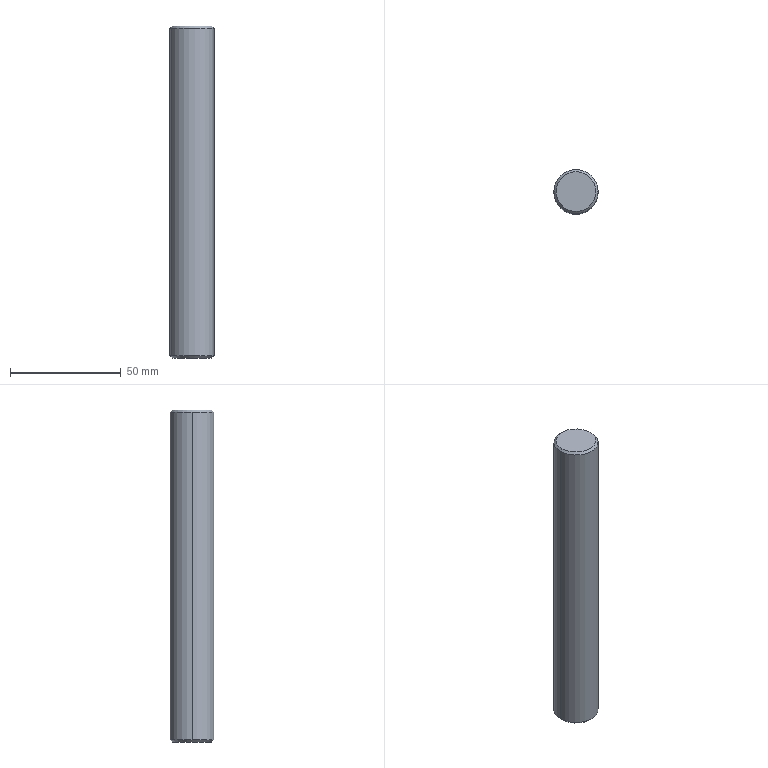Part | SolidWorks | features Chamfer 1, Extrusion 1 | 1 solid | 8 faces | box 20 x 20 x 150 mm | volume 47063 mm3 | cone 4 | cylinder 2 | plane 2 | commonest cylinder face diameters 20 x2
STEP:
#1=CARTESIAN_POINT('',(9.,0.,0.));
#2=VERTEX_POINT('',#1);
#3=CARTESIAN_POINT('',(-9.,0.,0.));
#4=VERTEX_POINT('',#3);
#5=CARTESIAN_POINT('',(0.,0.,0.));
#6=DIRECTION('',(0.,0.,1.));
#7=DIRECTION('',(1.,0.,0.));
#8=AXIS2_PLACEMENT_3D('',#5,#6,#7);
#9=CIRCLE('',#8,9.);
#10=EDGE_CURVE('',#2,#4,#9,.T.);
#11=ORIENTED_EDGE('',*,*,#10,.F.);
#12=CARTESIAN_POINT('',(10.,0.,-1.));
#13=VERTEX_POINT('',#12);
#14=CARTESIAN_POINT('',(9.,0.,0.));
#15=DIRECTION('',(0.7071,0.,-0.7071));
#16=VECTOR('',#15,1000.);
#17=LINE('',#14,#16);
#18=EDGE_CURVE('',#2,#13,#17,.T.);
#19=ORIENTED_EDGE('',*,*,#18,.T.);
#20=CARTESIAN_POINT('',(-10.,0.,-1.));
#21=VERTEX_POINT('',#20);
#22=CARTESIAN_POINT('',(0.,0.,-1.));
#23=DIRECTION('',(0.,0.,-1.));
#24=DIRECTION('',(1.,0.,0.));
#25=AXIS2_PLACEMENT_3D('',#22,#23,#24);
#26=CIRCLE('',#25,10.);
#27=EDGE_CURVE('',#21,#13,#26,.T.);
#28=ORIENTED_EDGE('',*,*,#27,.F.);
#29=CARTESIAN_POINT('',(-9.,0.,0.));
#30=DIRECTION('',(-0.7071,0.,-0.7071));
#31=VECTOR('',#30,1000.);
#32=LINE('',#29,#31);
#33=EDGE_CURVE('',#4,#21,#32,.T.);
#34=ORIENTED_EDGE('',*,*,#33,.F.);
#35=EDGE_LOOP('',(#11,#19,#28,#34));
#36=FACE_OUTER_BOUND('',#35,.T.);
#37=CARTESIAN_POINT('',(0.,0.,0.));
#38=DIRECTION('',(0.,0.,-1.));
#39=DIRECTION('',(-1.,0.,0.));
#40=AXIS2_PLACEMENT_3D('',#37,#38,#39);
#41=CONICAL_SURFACE('',#40,9.,0.7854);
#42=ADVANCED_FACE('',(#36),#41,.T.);
#43=CARTESIAN_POINT('',(-9.,0.,-150.));
#44=VERTEX_POINT('',#43);
#45=CARTESIAN_POINT('',(9.,0.,-150.));
#46=VERTEX_POINT('',#45);
#47=CARTESIAN_POINT('',(0.,0.,-150.));
#48=DIRECTION('',(0.,0.,-1.));
#49=DIRECTION('',(1.,0.,0.));
#50=AXIS2_PLACEMENT_3D('',#47,#48,#49);
#51=CIRCLE('',#50,9.);
#52=EDGE_CURVE('',#44,#46,#51,.T.);
#53=ORIENTED_EDGE('',*,*,#52,.F.);
#54=CARTESIAN_POINT('',(-10.,0.,-149.));
#55=VERTEX_POINT('',#54);
#56=CARTESIAN_POINT('',(-10.,0.,-149.));
#57=DIRECTION('',(-0.7071,0.,0.7071));
#58=VECTOR('',#57,1000.);
#59=LINE('',#56,#58);
#60=EDGE_CURVE('',#44,#55,#59,.T.);
#61=ORIENTED_EDGE('',*,*,#60,.T.);
#62=CARTESIAN_POINT('',(10.,0.,-149.));
#63=VERTEX_POINT('',#62);
#64=CARTESIAN_POINT('',(0.,0.,-149.));
#65=DIRECTION('',(0.,0.,1.));
#66=DIRECTION('',(1.,0.,0.));
#67=AXIS2_PLACEMENT_3D('',#64,#65,#66);
#68=CIRCLE('',#67,10.);
#69=EDGE_CURVE('',#63,#55,#68,.T.);
#70=ORIENTED_EDGE('',*,*,#69,.F.);
#71=CARTESIAN_POINT('',(10.,0.,-149.));
#72=DIRECTION('',(0.7071,0.,0.7071));
#73=VECTOR('',#72,1000.);
#74=LINE('',#71,#73);
#75=EDGE_CURVE('',#46,#63,#74,.T.);
#76=ORIENTED_EDGE('',*,*,#75,.F.);
#77=EDGE_LOOP('',(#53,#61,#70,#76));
#78=FACE_OUTER_BOUND('',#77,.T.);
#79=CARTESIAN_POINT('',(0.,0.,-149.));
#80=DIRECTION('',(0.,0.,1.));
#81=DIRECTION('',(1.,0.,0.));
#82=AXIS2_PLACEMENT_3D('',#79,#80,#81);
#83=CONICAL_SURFACE('',#82,10.,0.7854);
#84=ADVANCED_FACE('',(#78),#83,.T.);
#85=ORIENTED_EDGE('',*,*,#69,.T.);
#86=CARTESIAN_POINT('',(-10.,0.,-150.));
#87=DIRECTION('',(0.,0.,1.));
#88=VECTOR('',#87,1000.);
#89=LINE('',#86,#88);
#90=EDGE_CURVE('',#55,#21,#89,.T.);
#91=ORIENTED_EDGE('',*,*,#90,.T.);
#92=ORIENTED_EDGE('',*,*,#27,.T.);
#93=CARTESIAN_POINT('',(10.,0.,-150.));
#94=DIRECTION('',(0.,0.,1.));
#95=VECTOR('',#94,1000.);
#96=LINE('',#93,#95);
#97=EDGE_CURVE('',#63,#13,#96,.T.);
#98=ORIENTED_EDGE('',*,*,#97,.F.);
#99=EDGE_LOOP('',(#85,#91,#92,#98));
#100=FACE_OUTER_BOUND('',#99,.T.);
#101=CARTESIAN_POINT('',(0.,0.,-150.));
#102=DIRECTION('',(0.,0.,1.));
#103=DIRECTION('',(1.,0.,0.));
#104=AXIS2_PLACEMENT_3D('',#101,#102,#103);
#105=CYLINDRICAL_SURFACE('',#104,10.);
#106=ADVANCED_FACE('',(#100),#105,.T.);
#107=ORIENTED_EDGE('',*,*,#90,.F.);
#108=CARTESIAN_POINT('',(0.,0.,-149.));
#109=DIRECTION('',(0.,0.,1.));
#110=DIRECTION('',(1.,0.,0.));
#111=AXIS2_PLACEMENT_3D('',#108,#109,#110);
#112=CIRCLE('',#111,10.);
#113=EDGE_CURVE('',#55,#63,#112,.T.);
#114=ORIENTED_EDGE('',*,*,#113,.T.);
#115=ORIENTED_EDGE('',*,*,#97,.T.);
#116=CARTESIAN_POINT('',(0.,0.,-1.));
#117=DIRECTION('',(0.,0.,-1.));
#118=DIRECTION('',(1.,0.,0.));
#119=AXIS2_PLACEMENT_3D('',#116,#117,#118);
#120=CIRCLE('',#119,10.);
#121=EDGE_CURVE('',#13,#21,#120,.T.);
#122=ORIENTED_EDGE('',*,*,#121,.T.);
#123=EDGE_LOOP('',(#107,#114,#115,#122));
#124=FACE_OUTER_BOUND('',#123,.T.);
#125=CARTESIAN_POINT('',(0.,0.,-150.));
#126=DIRECTION('',(0.,0.,1.));
#127=DIRECTION('',(1.,0.,0.));
#128=AXIS2_PLACEMENT_3D('',#125,#126,#127);
#129=CYLINDRICAL_SURFACE('',#128,10.);
#130=ADVANCED_FACE('',(#124),#129,.T.);
#131=CARTESIAN_POINT('',(0.,0.,-150.));
#132=DIRECTION('',(0.,0.,-1.));
#133=DIRECTION('',(1.,0.,0.));
#134=AXIS2_PLACEMENT_3D('',#131,#132,#133);
#135=CIRCLE('',#134,9.);
#136=EDGE_CURVE('',#46,#44,#135,.T.);
#137=ORIENTED_EDGE('',*,*,#136,.T.);
#138=ORIENTED_EDGE('',*,*,#52,.T.);
#139=EDGE_LOOP('',(#137,#138));
#140=FACE_OUTER_BOUND('',#139,.T.);
#141=CARTESIAN_POINT('',(0.,0.,-150.));
#142=DIRECTION('',(0.,0.,1.));
#143=DIRECTION('',(1.,0.,0.));
#144=AXIS2_PLACEMENT_3D('',#141,#142,#143);
#145=PLANE('',#144);
#146=ADVANCED_FACE('',(#140),#145,.F.);
#147=CARTESIAN_POINT('',(0.,0.,0.));
#148=DIRECTION('',(0.,0.,1.));
#149=DIRECTION('',(1.,0.,0.));
#150=AXIS2_PLACEMENT_3D('',#147,#148,#149);
#151=CIRCLE('',#150,9.);
#152=EDGE_CURVE('',#4,#2,#151,.T.);
#153=ORIENTED_EDGE('',*,*,#152,.T.);
#154=ORIENTED_EDGE('',*,*,#10,.T.);
#155=EDGE_LOOP('',(#153,#154));
#156=FACE_OUTER_BOUND('',#155,.T.);
#157=CARTESIAN_POINT('',(0.,0.,0.));
#158=DIRECTION('',(0.,0.,1.));
#159=DIRECTION('',(1.,0.,0.));
#160=AXIS2_PLACEMENT_3D('',#157,#158,#159);
#161=PLANE('',#160);
#162=ADVANCED_FACE('',(#156),#161,.T.);
#163=ORIENTED_EDGE('',*,*,#60,.F.);
#164=ORIENTED_EDGE('',*,*,#136,.F.);
#165=ORIENTED_EDGE('',*,*,#75,.T.);
#166=ORIENTED_EDGE('',*,*,#113,.F.);
#167=EDGE_LOOP('',(#163,#164,#165,#166));
#168=FACE_OUTER_BOUND('',#167,.T.);
#169=CARTESIAN_POINT('',(0.,0.,-149.));
#170=DIRECTION('',(0.,0.,1.));
#171=DIRECTION('',(1.,0.,0.));
#172=AXIS2_PLACEMENT_3D('',#169,#170,#171);
#173=CONICAL_SURFACE('',#172,10.,0.7854);
#174=ADVANCED_FACE('',(#168),#173,.T.);
#175=ORIENTED_EDGE('',*,*,#18,.F.);
#176=ORIENTED_EDGE('',*,*,#152,.F.);
#177=ORIENTED_EDGE('',*,*,#33,.T.);
#178=ORIENTED_EDGE('',*,*,#121,.F.);
#179=EDGE_LOOP('',(#175,#176,#177,#178));
#180=FACE_OUTER_BOUND('',#179,.T.);
#181=CARTESIAN_POINT('',(0.,0.,0.));
#182=DIRECTION('',(0.,0.,-1.));
#183=DIRECTION('',(-1.,0.,0.));
#184=AXIS2_PLACEMENT_3D('',#181,#182,#183);
#185=CONICAL_SURFACE('',#184,9.,0.7854);
#186=ADVANCED_FACE('',(#180),#185,.T.);
#187=CLOSED_SHELL('',(#42,#84,#106,#130,#146,#162,#174,#186));
#188=MANIFOLD_SOLID_BREP('',#187);
#189=CARTESIAN_POINT('',(0.,0.,0.));
#190=DIRECTION('',(0.,0.,1.));
#191=DIRECTION('',(1.,0.,0.));
#192=AXIS2_PLACEMENT_3D('',#189,#190,#191);
#193=(LENGTH_UNIT()NAMED_UNIT(*)SI_UNIT(.MILLI.,.METRE.));
#194=UNCERTAINTY_MEASURE_WITH_UNIT(LENGTH_MEASURE(0.00001),#193,'','');
#195=(NAMED_UNIT(*)PLANE_ANGLE_UNIT()SI_UNIT($,.RADIAN.));
#196=(NAMED_UNIT(*)SI_UNIT($,.STERADIAN.)SOLID_ANGLE_UNIT());
#197=(GEOMETRIC_REPRESENTATION_CONTEXT(3)GLOBAL_UNCERTAINTY_ASSIGNED_CONTEXT((#194))GLOBAL_UNIT_ASSIGNED_CONTEXT((#193,#195,#196))REPRESENTATION_CONTEXT('',''));
#198=ADVANCED_BREP_SHAPE_REPRESENTATION('',(#188,#192),#197);